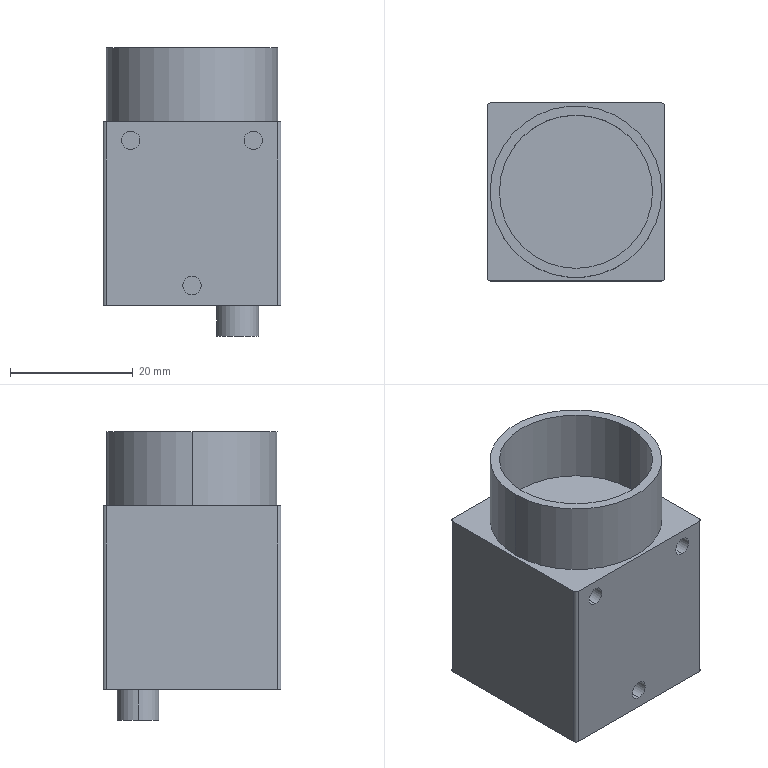Part | STEP file | ASND-0110-PG Flea2 | 1 solid | 28 faces | box 29 x 29 x 47.1 mm | volume 26811 mm3 | cylinder 16 | plane 12 | commonest cylinder face diameters 3 x6 1 x4 6.822 x2 25 x2 28 x2